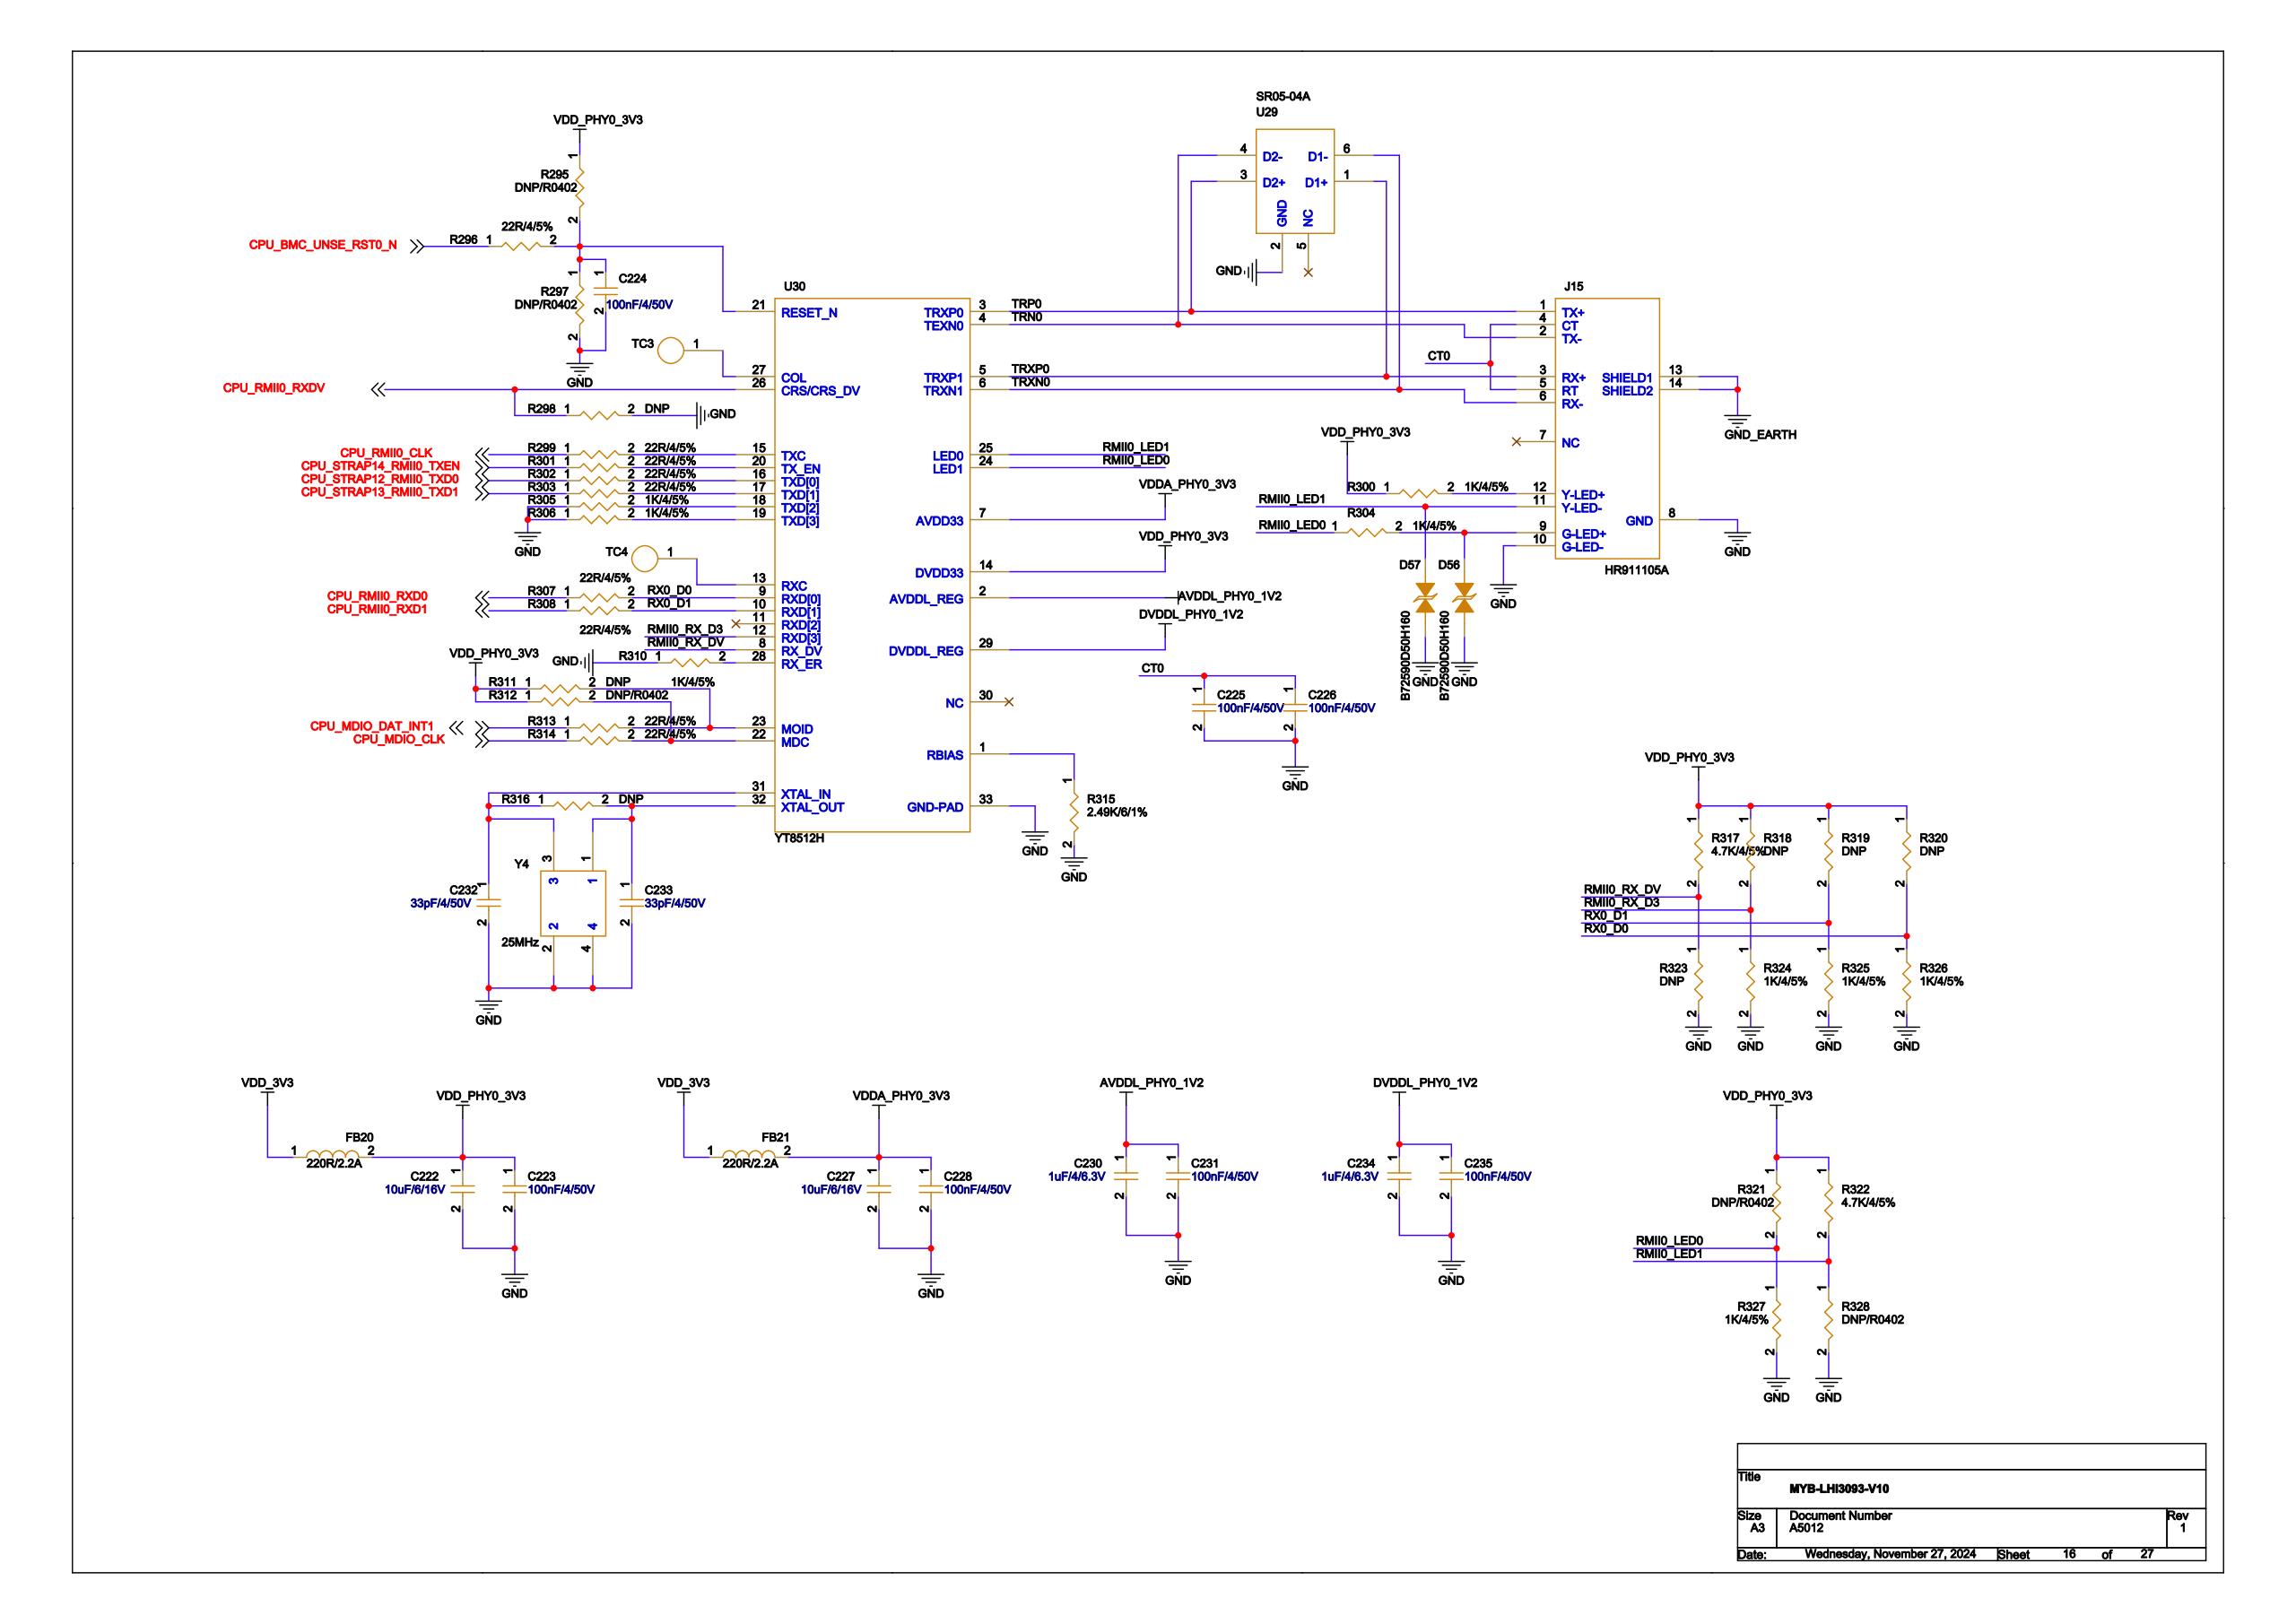Circuit board | Cadence Allegro | 1159 parts | 708 nets | one sheet of the schematic
Parts on this sheet (reference | value | footprint):
C222 | 10uF/6/16V | C0603
C223 | 100nF/4/50V | C0402
C224 | 100nF/4/50V | C0402
C225 | 100nF/4/50V | C0402
C226 | 100nF/4/50V | C0402
C227 | 10uF/6/16V | C0603
C228 | 100nF/4/50V | C0402
C230 | 1uF/4/6.3V | C0402
C231 | 100nF/4/50V | C0402
C232 | 33pF/4/50V | C0402
C233 | 33pF/4/50V | C0402
C234 | 1uF/4/6.3V | C0402
C235 | 100nF/4/50V | C0402
D56 | B72590D50H160 | D0402
FB20 | 220R/2.2A | FB0603
FB21 | 220R/2.2A | FB0603
J15 | HR911105A | RJ45-HR91105A
R295 | DNP/R0402 | R0402
R296 | 22R/4/5% | R0402
R297 | DNP/R0402 | R0402
R298 | DNP | R0402
R300 | 1K/4/5% | R0402
R301 | 22R/4/5% | R0402
R302 | 22R/4/5% | R0402
R303 | 22R/4/5% | R0402
R304 | 1K/4/5% | R0402
R305 | 1K/4/5% | R0402
R306 | 1K/4/5% | R0402
R307 | 22R/4/5% | R0402
R308 | 22R/4/5% | R0402
R310 | 1K/4/5% | R0402
R311 | DNP | R0402
R312 | DNP/R0402 | R0402
R313 | 22R/4/5% | R0402
R314 | 22R/4/5% | R0402
R315 | 2.49K/6/1% | R0402
R316 | DNP | R0402
R317 | 4.7K/4/5% | R0402
R318 | DNP | R0402
R319 | DNP | R0402
R320 | DNP | R0402
R321 | DNP/R0402 | R0402
R322 | 4.7K/4/5% | R0402
R323 | DNP | R0402
R324 | 1K/4/5% | R0402
R325 | 1K/4/5% | R0402
R326 | 1K/4/5% | R0402
R327 | 1K/4/5% | R0402
R328 | DNP/R0402 | R0402
TC3 | TP | TP_SMT
TC4 | TP | TP_SMT
U29 | SR05-04A | SOT23-6
U30 | YT8512H | QFN32
Y4 | 25MHz | 3225
Nets of these parts (net: part-pin ...):
GND: C222-2 C223-2 C224-2 C225-2 C226-2 C227-2 C228-2 C230-2 C231-2 C232-2 C233-2 C234-2 C235-2 D56-1 J15-8 J15-10 R297-2 R298-2 R305-1 R306-1 R310-1 R315-2 R323-2 R324-2 R325-2 R326-2 R327-2 R328-2 U29-2 Y4-2 Y4-4 U30-33
VDD_3V3: FB20-1 FB21-1
VDD_PHY0_3V3: C222-1 C223-1 FB20-2 R295-1 R300-1 R311-1 R312-1 R317-1 R318-1 R319-1 R320-1 R321-1 R322-1 U30-14
N15001496: C224-1 R295-2 R296-2 R297-1 U30-21
CT0: C225-1 C226-1 J15-4 J15-5
VDDA_PHY0_3V3: C227-1 C228-1 FB21-2 U30-7
AVDDL_PHY0_1V2: C230-1 C231-1 U30-2
DVDDL_PHY0_1V2: C234-1 C235-1 U30-29
GND_EARTH: J15-13 J15-14
N15012928: C232-1 R316-1 Y4-3 U30-31
N15012840: C233-1 R316-2 Y4-1 U30-32
N15015382: D56-2 J15-9 R304-2
RMII0_LED1: J15-11 R322-2 R328-1 U30-25
N15015306: J15-12 R300-2
RMII0_LED0: R304-1 R321-2 R327-1 U30-24
N15001115: R305-2 U30-18
N15001119: R306-2 U30-19
N15012138: R310-2 U30-28
RMII0_RX_D3: R318-2 R324-1 U30-12
RX0_D1: R308-2 R319-2 R325-1 U30-10
RX0_D0: R307-2 R320-2 R326-1 U30-9
CPU_MDIO_CLK: R314-1
CPU_MDIO_DAT_INT1: R313-1
CPU_BMC_UNSE_RST0_N: R296-1
CPU_STRAP14_RMII0_TXEN: R301-1
N15001103: R301-2 U30-20
CPU_STRAP12_RMII0_TXD0: R302-1
N15001107: R302-2 U30-16
CPU_STRAP13_RMII0_TXD1: R303-1
N15001111: R303-2 U30-17
CPU_RMII0_RXD0: R307-1
CPU_RMII0_RXD1: R308-1
N15012433: R311-2 R313-2 U30-23
N15012437: R312-2 R314-2 U30-22
RMII0_RX_DV: R317-2 R323-1 U30-8
CPU_RMII0_RXDV: R298-1 U30-26
N15013327: R315-1 U30-1
N15001437: TC3-1 U30-27
N15001424: TC4-1 U30-13
TRXP0: J15-3 U29-1 U30-5
TRXN0: J15-6 U29-6 U30-6
TRP0: J15-1 U29-3 U30-3
TRN0: J15-2 U29-4 U30-4